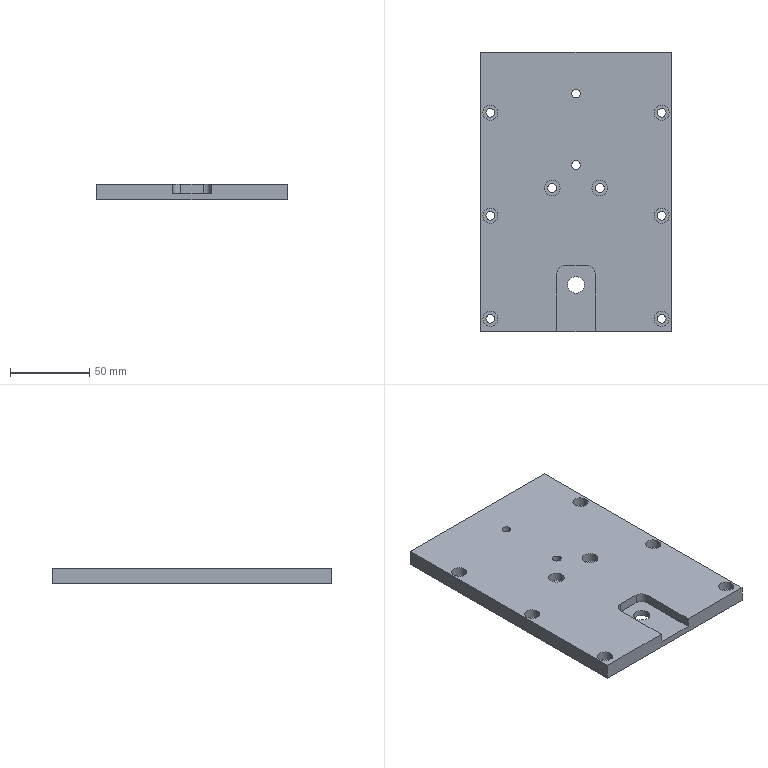Part | STEP file | 2045 Upper plate | 1 solid | 72 faces | box 120 x 176 x 10 mm | volume 199306 mm3 | cylinder 48 | plane 20 | cone 4 | commonest cylinder face diameters 5.5 x20 9.5 x12 10 x10 4.2 x4 10.5 x2